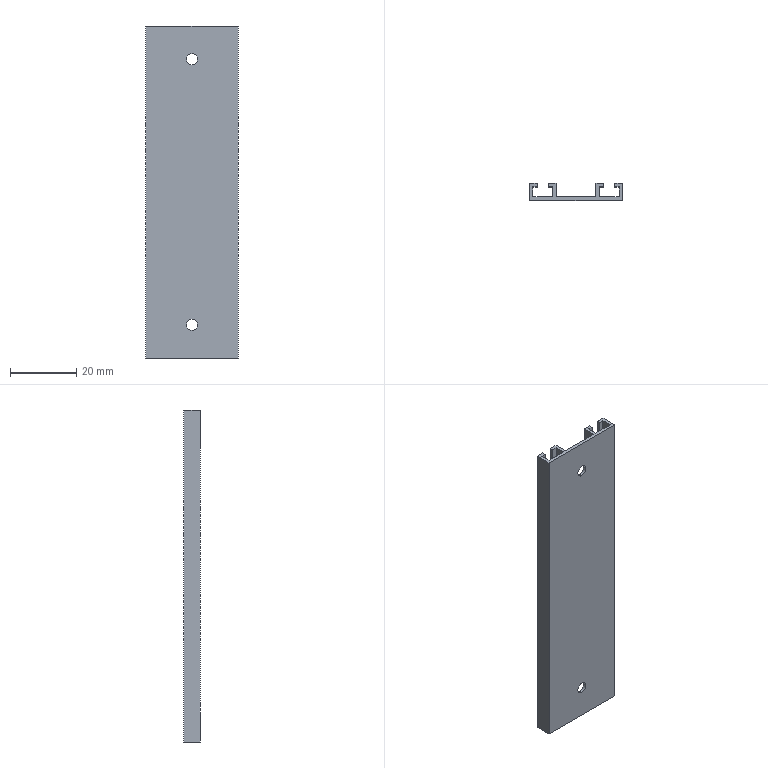Part | SolidWorks | features BossThin 1, ExtruThin 1, HoleWzd 1, MirrorSolid 1 | 1 solid | 30 faces | box 28 x 5 x 100 mm | volume 4922 mm3 | plane 26 | cylinder 4 | commonest cylinder face diameters 3.4 x4
STEP:
#1=CARTESIAN_POINT('',(-6.,0.,88.3));
#2=VERTEX_POINT('',#1);
#3=CARTESIAN_POINT('',(-6.,0.,91.7));
#4=VERTEX_POINT('',#3);
#5=CARTESIAN_POINT('',(-6.,0.,90.));
#6=DIRECTION('',(0.,1.,0.));
#7=DIRECTION('',(0.,0.,1.));
#8=AXIS2_PLACEMENT_3D('',#5,#6,#7);
#9=CIRCLE('',#8,1.7);
#10=EDGE_CURVE('',#2,#4,#9,.T.);
#11=ORIENTED_EDGE('',*,*,#10,.F.);
#12=CARTESIAN_POINT('',(-6.,1.,88.3));
#13=VERTEX_POINT('',#12);
#14=CARTESIAN_POINT('',(-6.,1.,88.3));
#15=DIRECTION('',(0.,1.,0.));
#16=VECTOR('',#15,1000.);
#17=LINE('',#14,#16);
#18=EDGE_CURVE('',#2,#13,#17,.T.);
#19=ORIENTED_EDGE('',*,*,#18,.T.);
#20=CARTESIAN_POINT('',(-6.,1.,91.7));
#21=VERTEX_POINT('',#20);
#22=CARTESIAN_POINT('',(-6.,1.,90.));
#23=DIRECTION('',(0.,1.,0.));
#24=DIRECTION('',(0.,0.,1.));
#25=AXIS2_PLACEMENT_3D('',#22,#23,#24);
#26=CIRCLE('',#25,1.7);
#27=EDGE_CURVE('',#13,#21,#26,.T.);
#28=ORIENTED_EDGE('',*,*,#27,.T.);
#29=CARTESIAN_POINT('',(-6.,1.,91.7));
#30=DIRECTION('',(0.,1.,0.));
#31=VECTOR('',#30,1000.);
#32=LINE('',#29,#31);
#33=EDGE_CURVE('',#4,#21,#32,.T.);
#34=ORIENTED_EDGE('',*,*,#33,.F.);
#35=EDGE_LOOP('',(#11,#19,#28,#34));
#36=FACE_OUTER_BOUND('',#35,.T.);
#37=CARTESIAN_POINT('',(-6.,1.,90.));
#38=DIRECTION('',(0.,1.,0.));
#39=DIRECTION('',(0.,0.,1.));
#40=AXIS2_PLACEMENT_3D('',#37,#38,#39);
#41=CYLINDRICAL_SURFACE('',#40,1.7);
#42=ADVANCED_FACE('',(#36),#41,.F.);
#43=CARTESIAN_POINT('',(-6.,0.,8.3));
#44=VERTEX_POINT('',#43);
#45=CARTESIAN_POINT('',(-6.,0.,11.7));
#46=VERTEX_POINT('',#45);
#47=CARTESIAN_POINT('',(-6.,0.,10.));
#48=DIRECTION('',(0.,1.,0.));
#49=DIRECTION('',(0.,0.,1.));
#50=AXIS2_PLACEMENT_3D('',#47,#48,#49);
#51=CIRCLE('',#50,1.7);
#52=EDGE_CURVE('',#44,#46,#51,.T.);
#53=ORIENTED_EDGE('',*,*,#52,.F.);
#54=CARTESIAN_POINT('',(-6.,1.,8.3));
#55=VERTEX_POINT('',#54);
#56=CARTESIAN_POINT('',(-6.,1.,8.3));
#57=DIRECTION('',(0.,1.,0.));
#58=VECTOR('',#57,1000.);
#59=LINE('',#56,#58);
#60=EDGE_CURVE('',#44,#55,#59,.T.);
#61=ORIENTED_EDGE('',*,*,#60,.T.);
#62=CARTESIAN_POINT('',(-6.,1.,11.7));
#63=VERTEX_POINT('',#62);
#64=CARTESIAN_POINT('',(-6.,1.,10.));
#65=DIRECTION('',(0.,1.,0.));
#66=DIRECTION('',(0.,0.,1.));
#67=AXIS2_PLACEMENT_3D('',#64,#65,#66);
#68=CIRCLE('',#67,1.7);
#69=EDGE_CURVE('',#55,#63,#68,.T.);
#70=ORIENTED_EDGE('',*,*,#69,.T.);
#71=CARTESIAN_POINT('',(-6.,1.,11.7));
#72=DIRECTION('',(0.,1.,0.));
#73=VECTOR('',#72,1000.);
#74=LINE('',#71,#73);
#75=EDGE_CURVE('',#46,#63,#74,.T.);
#76=ORIENTED_EDGE('',*,*,#75,.F.);
#77=EDGE_LOOP('',(#53,#61,#70,#76));
#78=FACE_OUTER_BOUND('',#77,.T.);
#79=CARTESIAN_POINT('',(-6.,1.,10.));
#80=DIRECTION('',(0.,1.,0.));
#81=DIRECTION('',(0.,0.,1.));
#82=AXIS2_PLACEMENT_3D('',#79,#80,#81);
#83=CYLINDRICAL_SURFACE('',#82,1.7);
#84=ADVANCED_FACE('',(#78),#83,.F.);
#85=CARTESIAN_POINT('',(0.,1.,0.));
#86=VERTEX_POINT('',#85);
#87=CARTESIAN_POINT('',(0.,5.,0.));
#88=VERTEX_POINT('',#87);
#89=CARTESIAN_POINT('',(0.,0.,0.));
#90=DIRECTION('',(0.,1.,0.));
#91=VECTOR('',#90,1000.);
#92=LINE('',#89,#91);
#93=EDGE_CURVE('',#86,#88,#92,.T.);
#94=ORIENTED_EDGE('',*,*,#93,.F.);
#95=CARTESIAN_POINT('',(0.,1.,100.));
#96=VERTEX_POINT('',#95);
#97=CARTESIAN_POINT('',(0.,1.,-6.083));
#98=DIRECTION('',(0.,0.,1.));
#99=VECTOR('',#98,1000.);
#100=LINE('',#97,#99);
#101=EDGE_CURVE('',#86,#96,#100,.T.);
#102=ORIENTED_EDGE('',*,*,#101,.T.);
#103=CARTESIAN_POINT('',(0.,5.,100.));
#104=VERTEX_POINT('',#103);
#105=CARTESIAN_POINT('',(0.,0.,100.));
#106=DIRECTION('',(0.,1.,0.));
#107=VECTOR('',#106,1000.);
#108=LINE('',#105,#107);
#109=EDGE_CURVE('',#96,#104,#108,.T.);
#110=ORIENTED_EDGE('',*,*,#109,.T.);
#111=CARTESIAN_POINT('',(0.,5.,100.));
#112=DIRECTION('',(0.,0.,-1.));
#113=VECTOR('',#112,1000.);
#114=LINE('',#111,#113);
#115=EDGE_CURVE('',#104,#88,#114,.T.);
#116=ORIENTED_EDGE('',*,*,#115,.T.);
#117=EDGE_LOOP('',(#94,#102,#110,#116));
#118=FACE_OUTER_BOUND('',#117,.T.);
#119=CARTESIAN_POINT('',(0.,0.,100.));
#120=DIRECTION('',(-1.,0.,0.));
#121=DIRECTION('',(0.,0.,1.));
#122=AXIS2_PLACEMENT_3D('',#119,#120,#121);
#123=PLANE('',#122);
#124=ADVANCED_FACE('',(#118),#123,.T.);
#125=CARTESIAN_POINT('',(1.,4.,0.));
#126=VERTEX_POINT('',#125);
#127=CARTESIAN_POINT('',(2.35,4.,0.));
#128=VERTEX_POINT('',#127);
#129=CARTESIAN_POINT('',(0.,4.,0.));
#130=DIRECTION('',(1.,0.,0.));
#131=VECTOR('',#130,1000.);
#132=LINE('',#129,#131);
#133=EDGE_CURVE('',#126,#128,#132,.T.);
#134=ORIENTED_EDGE('',*,*,#133,.T.);
#135=CARTESIAN_POINT('',(2.35,4.,100.));
#136=VERTEX_POINT('',#135);
#137=CARTESIAN_POINT('',(2.35,4.,100.));
#138=DIRECTION('',(0.,0.,-1.));
#139=VECTOR('',#138,1000.);
#140=LINE('',#137,#139);
#141=EDGE_CURVE('',#136,#128,#140,.T.);
#142=ORIENTED_EDGE('',*,*,#141,.F.);
#143=CARTESIAN_POINT('',(1.,4.,100.));
#144=VERTEX_POINT('',#143);
#145=CARTESIAN_POINT('',(0.,4.,100.));
#146=DIRECTION('',(1.,0.,0.));
#147=VECTOR('',#146,1000.);
#148=LINE('',#145,#147);
#149=EDGE_CURVE('',#144,#136,#148,.T.);
#150=ORIENTED_EDGE('',*,*,#149,.F.);
#151=CARTESIAN_POINT('',(1.,4.,100.));
#152=DIRECTION('',(0.,0.,-1.));
#153=VECTOR('',#152,1000.);
#154=LINE('',#151,#153);
#155=EDGE_CURVE('',#144,#126,#154,.T.);
#156=ORIENTED_EDGE('',*,*,#155,.T.);
#157=EDGE_LOOP('',(#134,#142,#150,#156));
#158=FACE_OUTER_BOUND('',#157,.T.);
#159=CARTESIAN_POINT('',(0.,4.,100.));
#160=DIRECTION('',(0.,1.,0.));
#161=DIRECTION('',(-1.,0.,0.));
#162=AXIS2_PLACEMENT_3D('',#159,#160,#161);
#163=PLANE('',#162);
#164=ADVANCED_FACE('',(#158),#163,.F.);
#165=CARTESIAN_POINT('',(2.35,5.,0.));
#166=VERTEX_POINT('',#165);
#167=CARTESIAN_POINT('',(2.35,5.,0.));
#168=DIRECTION('',(0.,-1.,0.));
#169=VECTOR('',#168,1000.);
#170=LINE('',#167,#169);
#171=EDGE_CURVE('',#166,#128,#170,.T.);
#172=ORIENTED_EDGE('',*,*,#171,.F.);
#173=CARTESIAN_POINT('',(2.35,5.,100.));
#174=VERTEX_POINT('',#173);
#175=CARTESIAN_POINT('',(2.35,5.,100.));
#176=DIRECTION('',(0.,0.,-1.));
#177=VECTOR('',#176,1000.);
#178=LINE('',#175,#177);
#179=EDGE_CURVE('',#174,#166,#178,.T.);
#180=ORIENTED_EDGE('',*,*,#179,.F.);
#181=CARTESIAN_POINT('',(2.35,5.,100.));
#182=DIRECTION('',(0.,-1.,0.));
#183=VECTOR('',#182,1000.);
#184=LINE('',#181,#183);
#185=EDGE_CURVE('',#174,#136,#184,.T.);
#186=ORIENTED_EDGE('',*,*,#185,.T.);
#187=ORIENTED_EDGE('',*,*,#141,.T.);
#188=EDGE_LOOP('',(#172,#180,#186,#187));
#189=FACE_OUTER_BOUND('',#188,.T.);
#190=CARTESIAN_POINT('',(2.35,5.,100.));
#191=DIRECTION('',(1.,0.,0.));
#192=DIRECTION('',(0.,1.,0.));
#193=AXIS2_PLACEMENT_3D('',#190,#191,#192);
#194=PLANE('',#193);
#195=ADVANCED_FACE('',(#189),#194,.T.);
#196=CARTESIAN_POINT('',(0.,5.,0.));
#197=DIRECTION('',(1.,0.,0.));
#198=VECTOR('',#197,1000.);
#199=LINE('',#196,#198);
#200=EDGE_CURVE('',#88,#166,#199,.T.);
#201=ORIENTED_EDGE('',*,*,#200,.F.);
#202=ORIENTED_EDGE('',*,*,#115,.F.);
#203=CARTESIAN_POINT('',(0.,5.,100.));
#204=DIRECTION('',(1.,0.,0.));
#205=VECTOR('',#204,1000.);
#206=LINE('',#203,#205);
#207=EDGE_CURVE('',#104,#174,#206,.T.);
#208=ORIENTED_EDGE('',*,*,#207,.T.);
#209=ORIENTED_EDGE('',*,*,#179,.T.);
#210=EDGE_LOOP('',(#201,#202,#208,#209));
#211=FACE_OUTER_BOUND('',#210,.T.);
#212=CARTESIAN_POINT('',(0.,5.,100.));
#213=DIRECTION('',(0.,1.,0.));
#214=DIRECTION('',(-1.,0.,0.));
#215=AXIS2_PLACEMENT_3D('',#212,#213,#214);
#216=PLANE('',#215);
#217=ADVANCED_FACE('',(#211),#216,.T.);
#218=CARTESIAN_POINT('',(-6.,0.,90.));
#219=DIRECTION('',(0.,1.,0.));
#220=DIRECTION('',(0.,0.,1.));
#221=AXIS2_PLACEMENT_3D('',#218,#219,#220);
#222=CIRCLE('',#221,1.7);
#223=EDGE_CURVE('',#4,#2,#222,.T.);
#224=ORIENTED_EDGE('',*,*,#223,.T.);
#225=ORIENTED_EDGE('',*,*,#10,.T.);
#226=EDGE_LOOP('',(#224,#225));
#227=FACE_BOUND('',#226,.T.);
#228=CARTESIAN_POINT('',(-6.,0.,10.));
#229=DIRECTION('',(0.,1.,0.));
#230=DIRECTION('',(0.,0.,1.));
#231=AXIS2_PLACEMENT_3D('',#228,#229,#230);
#232=CIRCLE('',#231,1.7);
#233=EDGE_CURVE('',#46,#44,#232,.T.);
#234=ORIENTED_EDGE('',*,*,#233,.T.);
#235=ORIENTED_EDGE('',*,*,#52,.T.);
#236=EDGE_LOOP('',(#234,#235));
#237=FACE_BOUND('',#236,.T.);
#238=CARTESIAN_POINT('',(8.,0.,0.));
#239=VERTEX_POINT('',#238);
#240=CARTESIAN_POINT('',(-20.,0.,0.));
#241=VERTEX_POINT('',#240);
#242=CARTESIAN_POINT('',(0.,0.,0.));
#243=DIRECTION('',(-1.,0.,0.));
#244=VECTOR('',#243,1000.);
#245=LINE('',#242,#244);
#246=EDGE_CURVE('',#239,#241,#245,.T.);
#247=ORIENTED_EDGE('',*,*,#246,.F.);
#248=CARTESIAN_POINT('',(8.,0.,100.));
#249=VERTEX_POINT('',#248);
#250=CARTESIAN_POINT('',(8.,0.,100.));
#251=DIRECTION('',(0.,0.,-1.));
#252=VECTOR('',#251,1000.);
#253=LINE('',#250,#252);
#254=EDGE_CURVE('',#249,#239,#253,.T.);
#255=ORIENTED_EDGE('',*,*,#254,.F.);
#256=CARTESIAN_POINT('',(-20.,0.,100.));
#257=VERTEX_POINT('',#256);
#258=CARTESIAN_POINT('',(0.,0.,100.));
#259=DIRECTION('',(-1.,0.,0.));
#260=VECTOR('',#259,1000.);
#261=LINE('',#258,#260);
#262=EDGE_CURVE('',#249,#257,#261,.T.);
#263=ORIENTED_EDGE('',*,*,#262,.T.);
#264=CARTESIAN_POINT('',(-20.,0.,100.));
#265=DIRECTION('',(0.,0.,-1.));
#266=VECTOR('',#265,1000.);
#267=LINE('',#264,#266);
#268=EDGE_CURVE('',#257,#241,#267,.T.);
#269=ORIENTED_EDGE('',*,*,#268,.T.);
#270=EDGE_LOOP('',(#247,#255,#263,#269));
#271=FACE_OUTER_BOUND('',#270,.T.);
#272=CARTESIAN_POINT('',(0.,0.,100.));
#273=DIRECTION('',(0.,-1.,0.));
#274=DIRECTION('',(0.,0.,-1.));
#275=AXIS2_PLACEMENT_3D('',#272,#273,#274);
#276=PLANE('',#275);
#277=ADVANCED_FACE('',(#227,#237,#271),#276,.T.);
#278=CARTESIAN_POINT('',(8.,5.,0.));
#279=VERTEX_POINT('',#278);
#280=CARTESIAN_POINT('',(8.,0.,0.));
#281=DIRECTION('',(0.,-1.,0.));
#282=VECTOR('',#281,1000.);
#283=LINE('',#280,#282);
#284=EDGE_CURVE('',#279,#239,#283,.T.);
#285=ORIENTED_EDGE('',*,*,#284,.F.);
#286=CARTESIAN_POINT('',(8.,5.,100.));
#287=VERTEX_POINT('',#286);
#288=CARTESIAN_POINT('',(8.,5.,100.));
#289=DIRECTION('',(0.,0.,-1.));
#290=VECTOR('',#289,1000.);
#291=LINE('',#288,#290);
#292=EDGE_CURVE('',#287,#279,#291,.T.);
#293=ORIENTED_EDGE('',*,*,#292,.F.);
#294=CARTESIAN_POINT('',(8.,0.,100.));
#295=DIRECTION('',(0.,-1.,0.));
#296=VECTOR('',#295,1000.);
#297=LINE('',#294,#296);
#298=EDGE_CURVE('',#287,#249,#297,.T.);
#299=ORIENTED_EDGE('',*,*,#298,.T.);
#300=ORIENTED_EDGE('',*,*,#254,.T.);
#301=EDGE_LOOP('',(#285,#293,#299,#300));
#302=FACE_OUTER_BOUND('',#301,.T.);
#303=CARTESIAN_POINT('',(8.,0.,100.));
#304=DIRECTION('',(1.,0.,0.));
#305=DIRECTION('',(0.,0.,-1.));
#306=AXIS2_PLACEMENT_3D('',#303,#304,#305);
#307=PLANE('',#306);
#308=ADVANCED_FACE('',(#302),#307,.T.);
#309=CARTESIAN_POINT('',(5.65,5.,0.));
#310=VERTEX_POINT('',#309);
#311=CARTESIAN_POINT('',(8.,5.,0.));
#312=DIRECTION('',(1.,0.,0.));
#313=VECTOR('',#312,1000.);
#314=LINE('',#311,#313);
#315=EDGE_CURVE('',#310,#279,#314,.T.);
#316=ORIENTED_EDGE('',*,*,#315,.F.);
#317=CARTESIAN_POINT('',(5.65,5.,100.));
#318=VERTEX_POINT('',#317);
#319=CARTESIAN_POINT('',(5.65,5.,100.));
#320=DIRECTION('',(0.,0.,-1.));
#321=VECTOR('',#320,1000.);
#322=LINE('',#319,#321);
#323=EDGE_CURVE('',#318,#310,#322,.T.);
#324=ORIENTED_EDGE('',*,*,#323,.F.);
#325=CARTESIAN_POINT('',(8.,5.,100.));
#326=DIRECTION('',(1.,0.,0.));
#327=VECTOR('',#326,1000.);
#328=LINE('',#325,#327);
#329=EDGE_CURVE('',#318,#287,#328,.T.);
#330=ORIENTED_EDGE('',*,*,#329,.T.);
#331=ORIENTED_EDGE('',*,*,#292,.T.);
#332=EDGE_LOOP('',(#316,#324,#330,#331));
#333=FACE_OUTER_BOUND('',#332,.T.);
#334=CARTESIAN_POINT('',(8.,5.,100.));
#335=DIRECTION('',(0.,1.,0.));
#336=DIRECTION('',(-1.,0.,0.));
#337=AXIS2_PLACEMENT_3D('',#334,#335,#336);
#338=PLANE('',#337);
#339=ADVANCED_FACE('',(#333),#338,.T.);
#340=CARTESIAN_POINT('',(5.65,4.,0.));
#341=VERTEX_POINT('',#340);
#342=CARTESIAN_POINT('',(5.65,4.,0.));
#343=DIRECTION('',(0.,1.,0.));
#344=VECTOR('',#343,1000.);
#345=LINE('',#342,#344);
#346=EDGE_CURVE('',#341,#310,#345,.T.);
#347=ORIENTED_EDGE('',*,*,#346,.F.);
#348=CARTESIAN_POINT('',(5.65,4.,100.));
#349=VERTEX_POINT('',#348);
#350=CARTESIAN_POINT('',(5.65,4.,100.));
#351=DIRECTION('',(0.,0.,-1.));
#352=VECTOR('',#351,1000.);
#353=LINE('',#350,#352);
#354=EDGE_CURVE('',#349,#341,#353,.T.);
#355=ORIENTED_EDGE('',*,*,#354,.F.);
#356=CARTESIAN_POINT('',(5.65,4.,100.));
#357=DIRECTION('',(0.,1.,0.));
#358=VECTOR('',#357,1000.);
#359=LINE('',#356,#358);
#360=EDGE_CURVE('',#349,#318,#359,.T.);
#361=ORIENTED_EDGE('',*,*,#360,.T.);
#362=ORIENTED_EDGE('',*,*,#323,.T.);
#363=EDGE_LOOP('',(#347,#355,#361,#362));
#364=FACE_OUTER_BOUND('',#363,.T.);
#365=CARTESIAN_POINT('',(5.65,4.,100.));
#366=DIRECTION('',(-1.,0.,0.));
#367=DIRECTION('',(0.,0.,1.));
#368=AXIS2_PLACEMENT_3D('',#365,#366,#367);
#369=PLANE('',#368);
#370=ADVANCED_FACE('',(#364),#369,.T.);
#371=CARTESIAN_POINT('',(7.,4.,0.));
#372=VERTEX_POINT('',#371);
#373=CARTESIAN_POINT('',(8.,4.,0.));
#374=DIRECTION('',(1.,0.,0.));
#375=VECTOR('',#374,1000.);
#376=LINE('',#373,#375);
#377=EDGE_CURVE('',#341,#372,#376,.T.);
#378=ORIENTED_EDGE('',*,*,#377,.T.);
#379=CARTESIAN_POINT('',(7.,4.,100.));
#380=VERTEX_POINT('',#379);
#381=CARTESIAN_POINT('',(7.,4.,100.));
#382=DIRECTION('',(0.,0.,-1.));
#383=VECTOR('',#382,1000.);
#384=LINE('',#381,#383);
#385=EDGE_CURVE('',#380,#372,#384,.T.);
#386=ORIENTED_EDGE('',*,*,#385,.F.);
#387=CARTESIAN_POINT('',(8.,4.,100.));
#388=DIRECTION('',(1.,0.,0.));
#389=VECTOR('',#388,1000.);
#390=LINE('',#387,#389);
#391=EDGE_CURVE('',#349,#380,#390,.T.);
#392=ORIENTED_EDGE('',*,*,#391,.F.);
#393=ORIENTED_EDGE('',*,*,#354,.T.);
#394=EDGE_LOOP('',(#378,#386,#392,#393));
#395=FACE_OUTER_BOUND('',#394,.T.);
#396=CARTESIAN_POINT('',(8.,4.,100.));
#397=DIRECTION('',(0.,1.,0.));
#398=DIRECTION('',(-1.,0.,0.));
#399=AXIS2_PLACEMENT_3D('',#396,#397,#398);
#400=PLANE('',#399);
#401=ADVANCED_FACE('',(#395),#400,.F.);
#402=CARTESIAN_POINT('',(7.,1.,0.));
#403=VERTEX_POINT('',#402);
#404=CARTESIAN_POINT('',(7.,0.,0.));
#405=DIRECTION('',(0.,-1.,0.));
#406=VECTOR('',#405,1000.);
#407=LINE('',#404,#406);
#408=EDGE_CURVE('',#372,#403,#407,.T.);
#409=ORIENTED_EDGE('',*,*,#408,.T.);
#410=CARTESIAN_POINT('',(7.,1.,100.));
#411=VERTEX_POINT('',#410);
#412=CARTESIAN_POINT('',(7.,1.,100.));
#413=DIRECTION('',(0.,0.,-1.));
#414=VECTOR('',#413,1000.);
#415=LINE('',#412,#414);
#416=EDGE_CURVE('',#411,#403,#415,.T.);
#417=ORIENTED_EDGE('',*,*,#416,.F.);
#418=CARTESIAN_POINT('',(7.,0.,100.));
#419=DIRECTION('',(0.,-1.,0.));
#420=VECTOR('',#419,1000.);
#421=LINE('',#418,#420);
#422=EDGE_CURVE('',#380,#411,#421,.T.);
#423=ORIENTED_EDGE('',*,*,#422,.F.);
#424=ORIENTED_EDGE('',*,*,#385,.T.);
#425=EDGE_LOOP('',(#409,#417,#423,#424));
#426=FACE_OUTER_BOUND('',#425,.T.);
#427=CARTESIAN_POINT('',(7.,0.,100.));
#428=DIRECTION('',(1.,0.,0.));
#429=DIRECTION('',(0.,0.,-1.));
#430=AXIS2_PLACEMENT_3D('',#427,#428,#429);
#431=PLANE('',#430);
#432=ADVANCED_FACE('',(#426),#431,.F.);
#433=CARTESIAN_POINT('',(1.,1.,0.));
#434=VERTEX_POINT('',#433);
#435=CARTESIAN_POINT('',(0.,1.,0.));
#436=DIRECTION('',(-1.,0.,0.));
#437=VECTOR('',#436,1000.);
#438=LINE('',#435,#437);
#439=EDGE_CURVE('',#403,#434,#438,.T.);
#440=ORIENTED_EDGE('',*,*,#439,.T.);
#441=CARTESIAN_POINT('',(1.,1.,100.));
#442=VERTEX_POINT('',#441);
#443=CARTESIAN_POINT('',(1.,1.,100.));
#444=DIRECTION('',(0.,0.,-1.));
#445=VECTOR('',#444,1000.);
#446=LINE('',#443,#445);
#447=EDGE_CURVE('',#442,#434,#446,.T.);
#448=ORIENTED_EDGE('',*,*,#447,.F.);
#449=CARTESIAN_POINT('',(0.,1.,100.));
#450=DIRECTION('',(-1.,0.,0.));
#451=VECTOR('',#450,1000.);
#452=LINE('',#449,#451);
#453=EDGE_CURVE('',#411,#442,#452,.T.);
#454=ORIENTED_EDGE('',*,*,#453,.F.);
#455=ORIENTED_EDGE('',*,*,#416,.T.);
#456=EDGE_LOOP('',(#440,#448,#454,#455));
#457=FACE_OUTER_BOUND('',#456,.T.);
#458=CARTESIAN_POINT('',(0.,1.,100.));
#459=DIRECTION('',(0.,-1.,0.));
#460=DIRECTION('',(0.,0.,-1.));
#461=AXIS2_PLACEMENT_3D('',#458,#459,#460);
#462=PLANE('',#461);
#463=ADVANCED_FACE('',(#457),#462,.F.);
#464=CARTESIAN_POINT('',(1.,0.,0.));
#465=DIRECTION('',(0.,1.,0.));
#466=VECTOR('',#465,1000.);
#467=LINE('',#464,#466);
#468=EDGE_CURVE('',#434,#126,#467,.T.);
#469=ORIENTED_EDGE('',*,*,#468,.T.);
#470=ORIENTED_EDGE('',*,*,#155,.F.);
#471=CARTESIAN_POINT('',(1.,0.,100.));
#472=DIRECTION('',(0.,1.,0.));
#473=VECTOR('',#472,1000.);
#474=LINE('',#471,#473);
#475=EDGE_CURVE('',#442,#144,#474,.T.);
#476=ORIENTED_EDGE('',*,*,#475,.F.);
#477=ORIENTED_EDGE('',*,*,#447,.T.);
#478=EDGE_LOOP('',(#469,#470,#476,#477));
#479=FACE_OUTER_BOUND('',#478,.T.);
#480=CARTESIAN_POINT('',(1.,0.,100.));
#481=DIRECTION('',(-1.,0.,0.));
#482=DIRECTION('',(0.,0.,1.));
#483=AXIS2_PLACEMENT_3D('',#480,#481,#482);
#484=PLANE('',#483);
#485=ADVANCED_FACE('',(#479),#484,.F.);
#486=ORIENTED_EDGE('',*,*,#149,.T.);
#487=ORIENTED_EDGE('',*,*,#185,.F.);
#488=ORIENTED_EDGE('',*,*,#207,.F.);
#489=ORIENTED_EDGE('',*,*,#109,.F.);
#490=CARTESIAN_POINT('',(-12.,1.,100.));
#491=VERTEX_POINT('',#490);
#492=CARTESIAN_POINT('',(0.,1.,100.));
#493=DIRECTION('',(-1.,0.,0.));
#494=VECTOR('',#493,1000.);
#495=LINE('',#492,#494);
#496=EDGE_CURVE('',#96,#491,#495,.T.);
#497=ORIENTED_EDGE('',*,*,#496,.T.);
#498=CARTESIAN_POINT('',(-12.,5.,100.));
#499=VERTEX_POINT('',#498);
#500=CARTESIAN_POINT('',(-12.,0.,100.));
#501=DIRECTION('',(0.,1.,0.));
#502=VECTOR('',#501,1000.);
#503=LINE('',#500,#502);
#504=EDGE_CURVE('',#491,#499,#503,.T.);
#505=ORIENTED_EDGE('',*,*,#504,.T.);
#506=CARTESIAN_POINT('',(-14.35,5.,100.));
#507=VERTEX_POINT('',#506);
#508=CARTESIAN_POINT('',(-12.,5.,100.));
#509=DIRECTION('',(-1.,0.,0.));
#510=VECTOR('',#509,1000.);
#511=LINE('',#508,#510);
#512=EDGE_CURVE('',#499,#507,#511,.T.);
#513=ORIENTED_EDGE('',*,*,#512,.T.);
#514=CARTESIAN_POINT('',(-14.35,4.,100.));
#515=VERTEX_POINT('',#514);
#516=CARTESIAN_POINT('',(-14.35,5.,100.));
#517=DIRECTION('',(0.,-1.,0.));
#518=VECTOR('',#517,1000.);
#519=LINE('',#516,#518);
#520=EDGE_CURVE('',#507,#515,#519,.T.);
#521=ORIENTED_EDGE('',*,*,#520,.T.);
#522=CARTESIAN_POINT('',(-13.,4.,100.));
#523=VERTEX_POINT('',#522);
#524=CARTESIAN_POINT('',(-12.,4.,100.));
#525=DIRECTION('',(-1.,0.,0.));
#526=VECTOR('',#525,1000.);
#527=LINE('',#524,#526);
#528=EDGE_CURVE('',#523,#515,#527,.T.);
#529=ORIENTED_EDGE('',*,*,#528,.F.);
#530=CARTESIAN_POINT('',(-13.,1.,100.));
#531=VERTEX_POINT('',#530);
#532=CARTESIAN_POINT('',(-13.,0.,100.));
#533=DIRECTION('',(0.,1.,0.));
#534=VECTOR('',#533,1000.);
#535=LINE('',#532,#534);
#536=EDGE_CURVE('',#531,#523,#535,.T.);
#537=ORIENTED_EDGE('',*,*,#536,.F.);
#538=CARTESIAN_POINT('',(-19.,1.,100.));
#539=VERTEX_POINT('',#538);
#540=CARTESIAN_POINT('',(-12.,1.,100.));
#541=DIRECTION('',(1.,0.,0.));
#542=VECTOR('',#541,1000.);
#543=LINE('',#540,#542);
#544=EDGE_CURVE('',#539,#531,#543,.T.);
#545=ORIENTED_EDGE('',*,*,#544,.F.);
#546=CARTESIAN_POINT('',(-19.,4.,100.));
#547=VERTEX_POINT('',#546);
#548=CARTESIAN_POINT('',(-19.,0.,100.));
#549=DIRECTION('',(0.,-1.,0.));
#550=VECTOR('',#549,1000.);
#551=LINE('',#548,#550);
#552=EDGE_CURVE('',#547,#539,#551,.T.);
#553=ORIENTED_EDGE('',*,*,#552,.F.);
#554=CARTESIAN_POINT('',(-17.65,4.,100.));
#555=VERTEX_POINT('',#554);
#556=CARTESIAN_POINT('',(-20.,4.,100.));
#557=DIRECTION('',(-1.,0.,0.));
#558=VECTOR('',#557,1000.);
#559=LINE('',#556,#558);
#560=EDGE_CURVE('',#555,#547,#559,.T.);
#561=ORIENTED_EDGE('',*,*,#560,.F.);
#562=CARTESIAN_POINT('',(-17.65,5.,100.));
#563=VERTEX_POINT('',#562);
#564=CARTESIAN_POINT('',(-17.65,4.,100.));
#565=DIRECTION('',(0.,1.,0.));
#566=VECTOR('',#565,1000.);
#567=LINE('',#564,#566);
#568=EDGE_CURVE('',#555,#563,#567,.T.);
#569=ORIENTED_EDGE('',*,*,#568,.T.);
#570=CARTESIAN_POINT('',(-20.,5.,100.));
#571=VERTEX_POINT('',#570);
#572=CARTESIAN_POINT('',(-20.,5.,100.));
#573=DIRECTION('',(-1.,0.,0.));
#574=VECTOR('',#573,1000.);
#575=LINE('',#572,#574);
#576=EDGE_CURVE('',#563,#571,#575,.T.);
#577=ORIENTED_EDGE('',*,*,#576,.T.);
#578=CARTESIAN_POINT('',(-20.,0.,100.));
#579=DIRECTION('',(0.,-1.,0.));
#580=VECTOR('',#579,1000.);
#581=LINE('',#578,#580);
#582=EDGE_CURVE('',#571,#257,#581,.T.);
#583=ORIENTED_EDGE('',*,*,#582,.T.);
#584=ORIENTED_EDGE('',*,*,#262,.F.);
#585=ORIENTED_EDGE('',*,*,#298,.F.);
#586=ORIENTED_EDGE('',*,*,#329,.F.);
#587=ORIENTED_EDGE('',*,*,#360,.F.);
#588=ORIENTED_EDGE('',*,*,#391,.T.);
#589=ORIENTED_EDGE('',*,*,#422,.T.);
#590=ORIENTED_EDGE('',*,*,#453,.T.);
#591=ORIENTED_EDGE('',*,*,#475,.T.);
#592=EDGE_LOOP('',(#486,#487,#488,#489,#497,#505,#513,#521,#529,#537,#545,#553,#561,#569,#577,#583,#584,#585,#586,#587,#588,#589,#590,#591));
#593=FACE_OUTER_BOUND('',#592,.T.);
#594=CARTESIAN_POINT('',(0.,0.,100.));
#595=DIRECTION('',(0.,0.,-1.));
#596=DIRECTION('',(-1.,0.,0.));
#597=AXIS2_PLACEMENT_3D('',#594,#595,#596);
#598=PLANE('',#597);
#599=ADVANCED_FACE('',(#593),#598,.F.);
#600=ORIENTED_EDGE('',*,*,#133,.F.);
#601=ORIENTED_EDGE('',*,*,#468,.F.);
#602=ORIENTED_EDGE('',*,*,#439,.F.);
#603=ORIENTED_EDGE('',*,*,#408,.F.);
#604=ORIENTED_EDGE('',*,*,#377,.F.);
#605=ORIENTED_EDGE('',*,*,#346,.T.);
#606=ORIENTED_EDGE('',*,*,#315,.T.);
#607=ORIENTED_EDGE('',*,*,#284,.T.);
#608=ORIENTED_EDGE('',*,*,#246,.T.);
#609=CARTESIAN_POINT('',(-20.,5.,0.));
#610=VERTEX_POINT('',#609);
#611=CARTESIAN_POINT('',(-20.,0.,0.));
#612=DIRECTION('',(0.,-1.,0.));
#613=VECTOR('',#612,1000.);
#614=LINE('',#611,#613);
#615=EDGE_CURVE('',#610,#241,#614,.T.);
#616=ORIENTED_EDGE('',*,*,#615,.F.);
#617=CARTESIAN_POINT('',(-17.65,5.,0.));
#618=VERTEX_POINT('',#617);
#619=CARTESIAN_POINT('',(-20.,5.,0.));
#620=DIRECTION('',(-1.,0.,0.));
#621=VECTOR('',#620,1000.);
#622=LINE('',#619,#621);
#623=EDGE_CURVE('',#618,#610,#622,.T.);
#624=ORIENTED_EDGE('',*,*,#623,.F.);
#625=CARTESIAN_POINT('',(-17.65,4.,0.));
#626=VERTEX_POINT('',#625);
#627=CARTESIAN_POINT('',(-17.65,4.,0.));
#628=DIRECTION('',(0.,1.,0.));
#629=VECTOR('',#628,1000.);
#630=LINE('',#627,#629);
#631=EDGE_CURVE('',#626,#618,#630,.T.);
#632=ORIENTED_EDGE('',*,*,#631,.F.);
#633=CARTESIAN_POINT('',(-19.,4.,0.));
#634=VERTEX_POINT('',#633);
#635=CARTESIAN_POINT('',(-20.,4.,0.));
#636=DIRECTION('',(-1.,0.,0.));
#637=VECTOR('',#636,1000.);
#638=LINE('',#635,#637);
#639=EDGE_CURVE('',#626,#634,#638,.T.);
#640=ORIENTED_EDGE('',*,*,#639,.T.);
#641=CARTESIAN_POINT('',(-19.,1.,0.));
#642=VERTEX_POINT('',#641);
#643=CARTESIAN_POINT('',(-19.,0.,0.));
#644=DIRECTION('',(0.,-1.,0.));
#645=VECTOR('',#644,1000.);
#646=LINE('',#643,#645);
#647=EDGE_CURVE('',#634,#642,#646,.T.);
#648=ORIENTED_EDGE('',*,*,#647,.T.);
#649=CARTESIAN_POINT('',(-13.,1.,0.));
#650=VERTEX_POINT('',#649);
#651=CARTESIAN_POINT('',(-12.,1.,0.));
#652=DIRECTION('',(1.,0.,0.));
#653=VECTOR('',#652,1000.);
#654=LINE('',#651,#653);
#655=EDGE_CURVE('',#642,#650,#654,.T.);
#656=ORIENTED_EDGE('',*,*,#655,.T.);
#657=CARTESIAN_POINT('',(-13.,4.,0.));
#658=VERTEX_POINT('',#657);
#659=CARTESIAN_POINT('',(-13.,0.,0.));
#660=DIRECTION('',(0.,1.,0.));
#661=VECTOR('',#660,1000.);
#662=LINE('',#659,#661);
#663=EDGE_CURVE('',#650,#658,#662,.T.);
#664=ORIENTED_EDGE('',*,*,#663,.T.);
#665=CARTESIAN_POINT('',(-14.35,4.,0.));
#666=VERTEX_POINT('',#665);
#667=CARTESIAN_POINT('',(-12.,4.,0.));
#668=DIRECTION('',(-1.,0.,0.));
#669=VECTOR('',#668,1000.);
#670=LINE('',#667,#669);
#671=EDGE_CURVE('',#658,#666,#670,.T.);
#672=ORIENTED_EDGE('',*,*,#671,.T.);
#673=CARTESIAN_POINT('',(-14.35,5.,0.));
#674=VERTEX_POINT('',#673);
#675=CARTESIAN_POINT('',(-14.35,5.,0.));
#676=DIRECTION('',(0.,-1.,0.));
#677=VECTOR('',#676,1000.);
#678=LINE('',#675,#677);
#679=EDGE_CURVE('',#674,#666,#678,.T.);
#680=ORIENTED_EDGE('',*,*,#679,.F.);
#681=CARTESIAN_POINT('',(-12.,5.,0.));
#682=VERTEX_POINT('',#681);
#683=CARTESIAN_POINT('',(-12.,5.,0.));
#684=DIRECTION('',(-1.,0.,0.));
#685=VECTOR('',#684,1000.);
#686=LINE('',#683,#685);
#687=EDGE_CURVE('',#682,#674,#686,.T.);
#688=ORIENTED_EDGE('',*,*,#687,.F.);
#689=CARTESIAN_POINT('',(-12.,1.,0.));
#690=VERTEX_POINT('',#689);
#691=CARTESIAN_POINT('',(-12.,0.,0.));
#692=DIRECTION('',(0.,1.,0.));
#693=VECTOR('',#692,1000.);
#694=LINE('',#691,#693);
#695=EDGE_CURVE('',#690,#682,#694,.T.);
#696=ORIENTED_EDGE('',*,*,#695,.F.);
#697=CARTESIAN_POINT('',(0.,1.,0.));
#698=DIRECTION('',(-1.,0.,0.));
#699=VECTOR('',#698,1000.);
#700=LINE('',#697,#699);
#701=EDGE_CURVE('',#86,#690,#700,.T.);
#702=ORIENTED_EDGE('',*,*,#701,.F.);
#703=ORIENTED_EDGE('',*,*,#93,.T.);
#704=ORIENTED_EDGE('',*,*,#200,.T.);
#705=ORIENTED_EDGE('',*,*,#171,.T.);
#706=EDGE_LOOP('',(#600,#601,#602,#603,#604,#605,#606,#607,#608,#616,#624,#632,#640,#648,#656,#664,#672,#680,#688,#696,#702,#703,#704,#705));
#707=FACE_OUTER_BOUND('',#706,.T.);
#708=CARTESIAN_POINT('',(0.,0.,0.));
#709=DIRECTION('',(0.,0.,-1.));
#710=DIRECTION('',(-1.,0.,0.));
#711=AXIS2_PLACEMENT_3D('',#708,#709,#710);
#712=PLANE('',#711);
#713=ADVANCED_FACE('',(#707),#712,.T.);
#714=CARTESIAN_POINT('',(-6.,1.,90.));
#715=DIRECTION('',(0.,1.,0.));
#716=DIRECTION('',(0.,0.,1.));
#717=AXIS2_PLACEMENT_3D('',#714,#715,#716);
#718=CIRCLE('',#717,1.7);
#719=EDGE_CURVE('',#21,#13,#718,.T.);
#720=ORIENTED_EDGE('',*,*,#719,.F.);
#721=ORIENTED_EDGE('',*,*,#27,.F.);
#722=EDGE_LOOP('',(#720,#721));
#723=FACE_BOUND('',#722,.T.);
#724=CARTESIAN_POINT('',(-6.,1.,10.));
#725=DIRECTION('',(0.,1.,0.));
#726=DIRECTION('',(0.,0.,1.));
#727=AXIS2_PLACEMENT_3D('',#724,#725,#726);
#728=CIRCLE('',#727,1.7);
#729=EDGE_CURVE('',#63,#55,#728,.T.);
#730=ORIENTED_EDGE('',*,*,#729,.F.);
#731=ORIENTED_EDGE('',*,*,#69,.F.);
#732=EDGE_LOOP('',(#730,#731));
#733=FACE_BOUND('',#732,.T.);
#734=ORIENTED_EDGE('',*,*,#101,.F.);
#735=ORIENTED_EDGE('',*,*,#701,.T.);
#736=CARTESIAN_POINT('',(-12.,1.,-6.083));
#737=DIRECTION('',(0.,0.,1.));
#738=VECTOR('',#737,1000.);
#739=LINE('',#736,#738);
#740=EDGE_CURVE('',#690,#491,#739,.T.);
#741=ORIENTED_EDGE('',*,*,#740,.T.);
#742=ORIENTED_EDGE('',*,*,#496,.F.);
#743=EDGE_LOOP('',(#734,#735,#741,#742));
#744=FACE_OUTER_BOUND('',#743,.T.);
#745=CARTESIAN_POINT('',(0.,1.,-6.083));
#746=DIRECTION('',(0.,1.,0.));
#747=DIRECTION('',(-1.,0.,0.));
#748=AXIS2_PLACEMENT_3D('',#745,#746,#747);
#749=PLANE('',#748);
#750=ADVANCED_FACE('',(#723,#733,#744),#749,.T.);
#751=ORIENTED_EDGE('',*,*,#695,.T.);
#752=CARTESIAN_POINT('',(-12.,5.,100.));
#753=DIRECTION('',(0.,0.,-1.));
#754=VECTOR('',#753,1000.);
#755=LINE('',#752,#754);
#756=EDGE_CURVE('',#499,#682,#755,.T.);
#757=ORIENTED_EDGE('',*,*,#756,.F.);
#758=ORIENTED_EDGE('',*,*,#504,.F.);
#759=ORIENTED_EDGE('',*,*,#740,.F.);
#760=EDGE_LOOP('',(#751,#757,#758,#759));
#761=FACE_OUTER_BOUND('',#760,.T.);
#762=CARTESIAN_POINT('',(-12.,0.,100.));
#763=DIRECTION('',(1.,0.,0.));
#764=DIRECTION('',(0.,0.,1.));
#765=AXIS2_PLACEMENT_3D('',#762,#763,#764);
#766=PLANE('',#765);
#767=ADVANCED_FACE('',(#761),#766,.T.);
#768=ORIENTED_EDGE('',*,*,#671,.F.);
#769=CARTESIAN_POINT('',(-13.,4.,100.));
#770=DIRECTION('',(0.,0.,-1.));
#771=VECTOR('',#770,1000.);
#772=LINE('',#769,#771);
#773=EDGE_CURVE('',#523,#658,#772,.T.);
#774=ORIENTED_EDGE('',*,*,#773,.F.);
#775=ORIENTED_EDGE('',*,*,#528,.T.);
#776=CARTESIAN_POINT('',(-14.35,4.,100.));
#777=DIRECTION('',(0.,0.,-1.));
#778=VECTOR('',#777,1000.);
#779=LINE('',#776,#778);
#780=EDGE_CURVE('',#515,#666,#779,.T.);
#781=ORIENTED_EDGE('',*,*,#780,.T.);
#782=EDGE_LOOP('',(#768,#774,#775,#781));
#783=FACE_OUTER_BOUND('',#782,.T.);
#784=CARTESIAN_POINT('',(-12.,4.,100.));
#785=DIRECTION('',(0.,1.,0.));
#786=DIRECTION('',(1.,0.,0.));
#787=AXIS2_PLACEMENT_3D('',#784,#785,#786);
#788=PLANE('',#787);
#789=ADVANCED_FACE('',(#783),#788,.F.);
#790=ORIENTED_EDGE('',*,*,#679,.T.);
#791=ORIENTED_EDGE('',*,*,#780,.F.);
#792=ORIENTED_EDGE('',*,*,#520,.F.);
#793=CARTESIAN_POINT('',(-14.35,5.,100.));
#794=DIRECTION('',(0.,0.,-1.));
#795=VECTOR('',#794,1000.);
#796=LINE('',#793,#795);
#797=EDGE_CURVE('',#507,#674,#796,.T.);
#798=ORIENTED_EDGE('',*,*,#797,.T.);
#799=EDGE_LOOP('',(#790,#791,#792,#798));
#800=FACE_OUTER_BOUND('',#799,.T.);
#801=CARTESIAN_POINT('',(-14.35,5.,100.));
#802=DIRECTION('',(-1.,0.,0.));
#803=DIRECTION('',(0.,1.,0.));
#804=AXIS2_PLACEMENT_3D('',#801,#802,#803);
#805=PLANE('',#804);
#806=ADVANCED_FACE('',(#800),#805,.T.);
#807=ORIENTED_EDGE('',*,*,#687,.T.);
#808=ORIENTED_EDGE('',*,*,#797,.F.);
#809=ORIENTED_EDGE('',*,*,#512,.F.);
#810=ORIENTED_EDGE('',*,*,#756,.T.);
#811=EDGE_LOOP('',(#807,#808,#809,#810));
#812=FACE_OUTER_BOUND('',#811,.T.);
#813=CARTESIAN_POINT('',(-12.,5.,100.));
#814=DIRECTION('',(0.,1.,0.));
#815=DIRECTION('',(1.,0.,0.));
#816=AXIS2_PLACEMENT_3D('',#813,#814,#815);
#817=PLANE('',#816);
#818=ADVANCED_FACE('',(#812),#817,.T.);
#819=ORIENTED_EDGE('',*,*,#615,.T.);
#820=ORIENTED_EDGE('',*,*,#268,.F.);
#821=ORIENTED_EDGE('',*,*,#582,.F.);
#822=CARTESIAN_POINT('',(-20.,5.,100.));
#823=DIRECTION('',(0.,0.,-1.));
#824=VECTOR('',#823,1000.);
#825=LINE('',#822,#824);
#826=EDGE_CURVE('',#571,#610,#825,.T.);
#827=ORIENTED_EDGE('',*,*,#826,.T.);
#828=EDGE_LOOP('',(#819,#820,#821,#827));
#829=FACE_OUTER_BOUND('',#828,.T.);
#830=CARTESIAN_POINT('',(-20.,0.,100.));
#831=DIRECTION('',(-1.,0.,0.));
#832=DIRECTION('',(0.,0.,-1.));
#833=AXIS2_PLACEMENT_3D('',#830,#831,#832);
#834=PLANE('',#833);
#835=ADVANCED_FACE('',(#829),#834,.T.);
#836=ORIENTED_EDGE('',*,*,#623,.T.);
#837=ORIENTED_EDGE('',*,*,#826,.F.);
#838=ORIENTED_EDGE('',*,*,#576,.F.);
#839=CARTESIAN_POINT('',(-17.65,5.,100.));
#840=DIRECTION('',(0.,0.,-1.));
#841=VECTOR('',#840,1000.);
#842=LINE('',#839,#841);
#843=EDGE_CURVE('',#563,#618,#842,.T.);
#844=ORIENTED_EDGE('',*,*,#843,.T.);
#845=EDGE_LOOP('',(#836,#837,#838,#844));
#846=FACE_OUTER_BOUND('',#845,.T.);
#847=CARTESIAN_POINT('',(-20.,5.,100.));
#848=DIRECTION('',(0.,1.,0.));
#849=DIRECTION('',(1.,0.,0.));
#850=AXIS2_PLACEMENT_3D('',#847,#848,#849);
#851=PLANE('',#850);
#852=ADVANCED_FACE('',(#846),#851,.T.);
#853=ORIENTED_EDGE('',*,*,#631,.T.);
#854=ORIENTED_EDGE('',*,*,#843,.F.);
#855=ORIENTED_EDGE('',*,*,#568,.F.);
#856=CARTESIAN_POINT('',(-17.65,4.,100.));
#857=DIRECTION('',(0.,0.,-1.));
#858=VECTOR('',#857,1000.);
#859=LINE('',#856,#858);
#860=EDGE_CURVE('',#555,#626,#859,.T.);
#861=ORIENTED_EDGE('',*,*,#860,.T.);
#862=EDGE_LOOP('',(#853,#854,#855,#861));
#863=FACE_OUTER_BOUND('',#862,.T.);
#864=CARTESIAN_POINT('',(-17.65,4.,100.));
#865=DIRECTION('',(1.,0.,0.));
#866=DIRECTION('',(0.,0.,1.));
#867=AXIS2_PLACEMENT_3D('',#864,#865,#866);
#868=PLANE('',#867);
#869=ADVANCED_FACE('',(#863),#868,.T.);
#870=ORIENTED_EDGE('',*,*,#639,.F.);
#871=ORIENTED_EDGE('',*,*,#860,.F.);
#872=ORIENTED_EDGE('',*,*,#560,.T.);
#873=CARTESIAN_POINT('',(-19.,4.,100.));
#874=DIRECTION('',(0.,0.,-1.));
#875=VECTOR('',#874,1000.);
#876=LINE('',#873,#875);
#877=EDGE_CURVE('',#547,#634,#876,.T.);
#878=ORIENTED_EDGE('',*,*,#877,.T.);
#879=EDGE_LOOP('',(#870,#871,#872,#878));
#880=FACE_OUTER_BOUND('',#879,.T.);
#881=CARTESIAN_POINT('',(-20.,4.,100.));
#882=DIRECTION('',(0.,1.,0.));
#883=DIRECTION('',(1.,0.,0.));
#884=AXIS2_PLACEMENT_3D('',#881,#882,#883);
#885=PLANE('',#884);
#886=ADVANCED_FACE('',(#880),#885,.F.);
#887=ORIENTED_EDGE('',*,*,#647,.F.);
#888=ORIENTED_EDGE('',*,*,#877,.F.);
#889=ORIENTED_EDGE('',*,*,#552,.T.);
#890=CARTESIAN_POINT('',(-19.,1.,100.));
#891=DIRECTION('',(0.,0.,-1.));
#892=VECTOR('',#891,1000.);
#893=LINE('',#890,#892);
#894=EDGE_CURVE('',#539,#642,#893,.T.);
#895=ORIENTED_EDGE('',*,*,#894,.T.);
#896=EDGE_LOOP('',(#887,#888,#889,#895));
#897=FACE_OUTER_BOUND('',#896,.T.);
#898=CARTESIAN_POINT('',(-19.,0.,100.));
#899=DIRECTION('',(-1.,0.,0.));
#900=DIRECTION('',(0.,0.,-1.));
#901=AXIS2_PLACEMENT_3D('',#898,#899,#900);
#902=PLANE('',#901);
#903=ADVANCED_FACE('',(#897),#902,.F.);
#904=ORIENTED_EDGE('',*,*,#655,.F.);
#905=ORIENTED_EDGE('',*,*,#894,.F.);
#906=ORIENTED_EDGE('',*,*,#544,.T.);
#907=CARTESIAN_POINT('',(-13.,1.,100.));
#908=DIRECTION('',(0.,0.,-1.));
#909=VECTOR('',#908,1000.);
#910=LINE('',#907,#909);
#911=EDGE_CURVE('',#531,#650,#910,.T.);
#912=ORIENTED_EDGE('',*,*,#911,.T.);
#913=EDGE_LOOP('',(#904,#905,#906,#912));
#914=FACE_OUTER_BOUND('',#913,.T.);
#915=CARTESIAN_POINT('',(-12.,1.,100.));
#916=DIRECTION('',(0.,-1.,0.));
#917=DIRECTION('',(0.,0.,-1.));
#918=AXIS2_PLACEMENT_3D('',#915,#916,#917);
#919=PLANE('',#918);
#920=ADVANCED_FACE('',(#914),#919,.F.);
#921=ORIENTED_EDGE('',*,*,#663,.F.);
#922=ORIENTED_EDGE('',*,*,#911,.F.);
#923=ORIENTED_EDGE('',*,*,#536,.T.);
#924=ORIENTED_EDGE('',*,*,#773,.T.);
#925=EDGE_LOOP('',(#921,#922,#923,#924));
#926=FACE_OUTER_BOUND('',#925,.T.);
#927=CARTESIAN_POINT('',(-13.,0.,100.));
#928=DIRECTION('',(1.,0.,0.));
#929=DIRECTION('',(0.,0.,1.));
#930=AXIS2_PLACEMENT_3D('',#927,#928,#929);
#931=PLANE('',#930);
#932=ADVANCED_FACE('',(#926),#931,.F.);
#933=ORIENTED_EDGE('',*,*,#60,.F.);
#934=ORIENTED_EDGE('',*,*,#233,.F.);
#935=ORIENTED_EDGE('',*,*,#75,.T.);
#936=ORIENTED_EDGE('',*,*,#729,.T.);
#937=EDGE_LOOP('',(#933,#934,#935,#936));
#938=FACE_OUTER_BOUND('',#937,.T.);
#939=CARTESIAN_POINT('',(-6.,1.,10.));
#940=DIRECTION('',(0.,1.,0.));
#941=DIRECTION('',(0.,0.,1.));
#942=AXIS2_PLACEMENT_3D('',#939,#940,#941);
#943=CYLINDRICAL_SURFACE('',#942,1.7);
#944=ADVANCED_FACE('',(#938),#943,.F.);
#945=ORIENTED_EDGE('',*,*,#18,.F.);
#946=ORIENTED_EDGE('',*,*,#223,.F.);
#947=ORIENTED_EDGE('',*,*,#33,.T.);
#948=ORIENTED_EDGE('',*,*,#719,.T.);
#949=EDGE_LOOP('',(#945,#946,#947,#948));
#950=FACE_OUTER_BOUND('',#949,.T.);
#951=CARTESIAN_POINT('',(-6.,1.,90.));
#952=DIRECTION('',(0.,1.,0.));
#953=DIRECTION('',(0.,0.,1.));
#954=AXIS2_PLACEMENT_3D('',#951,#952,#953);
#955=CYLINDRICAL_SURFACE('',#954,1.7);
#956=ADVANCED_FACE('',(#950),#955,.F.);
#957=CLOSED_SHELL('',(#42,#84,#124,#164,#195,#217,#277,#308,#339,#370,#401,#432,#463,#485,#599,#713,#750,#767,#789,#806,#818,#835,#852,#869,#886,#903,#920,#932,#944,#956));
#958=MANIFOLD_SOLID_BREP('',#957);
#959=CARTESIAN_POINT('',(0.,0.,0.));
#960=DIRECTION('',(0.,0.,1.));
#961=DIRECTION('',(1.,0.,0.));
#962=AXIS2_PLACEMENT_3D('',#959,#960,#961);
#963=(LENGTH_UNIT()NAMED_UNIT(*)SI_UNIT(.MILLI.,.METRE.));
#964=UNCERTAINTY_MEASURE_WITH_UNIT(LENGTH_MEASURE(0.00001),#963,'','');
#965=(NAMED_UNIT(*)PLANE_ANGLE_UNIT()SI_UNIT($,.RADIAN.));
#966=(NAMED_UNIT(*)SI_UNIT($,.STERADIAN.)SOLID_ANGLE_UNIT());
#967=(GEOMETRIC_REPRESENTATION_CONTEXT(3)GLOBAL_UNCERTAINTY_ASSIGNED_CONTEXT((#964))GLOBAL_UNIT_ASSIGNED_CONTEXT((#963,#965,#966))REPRESENTATION_CONTEXT('',''));
#968=ADVANCED_BREP_SHAPE_REPRESENTATION('',(#958,#962),#967);